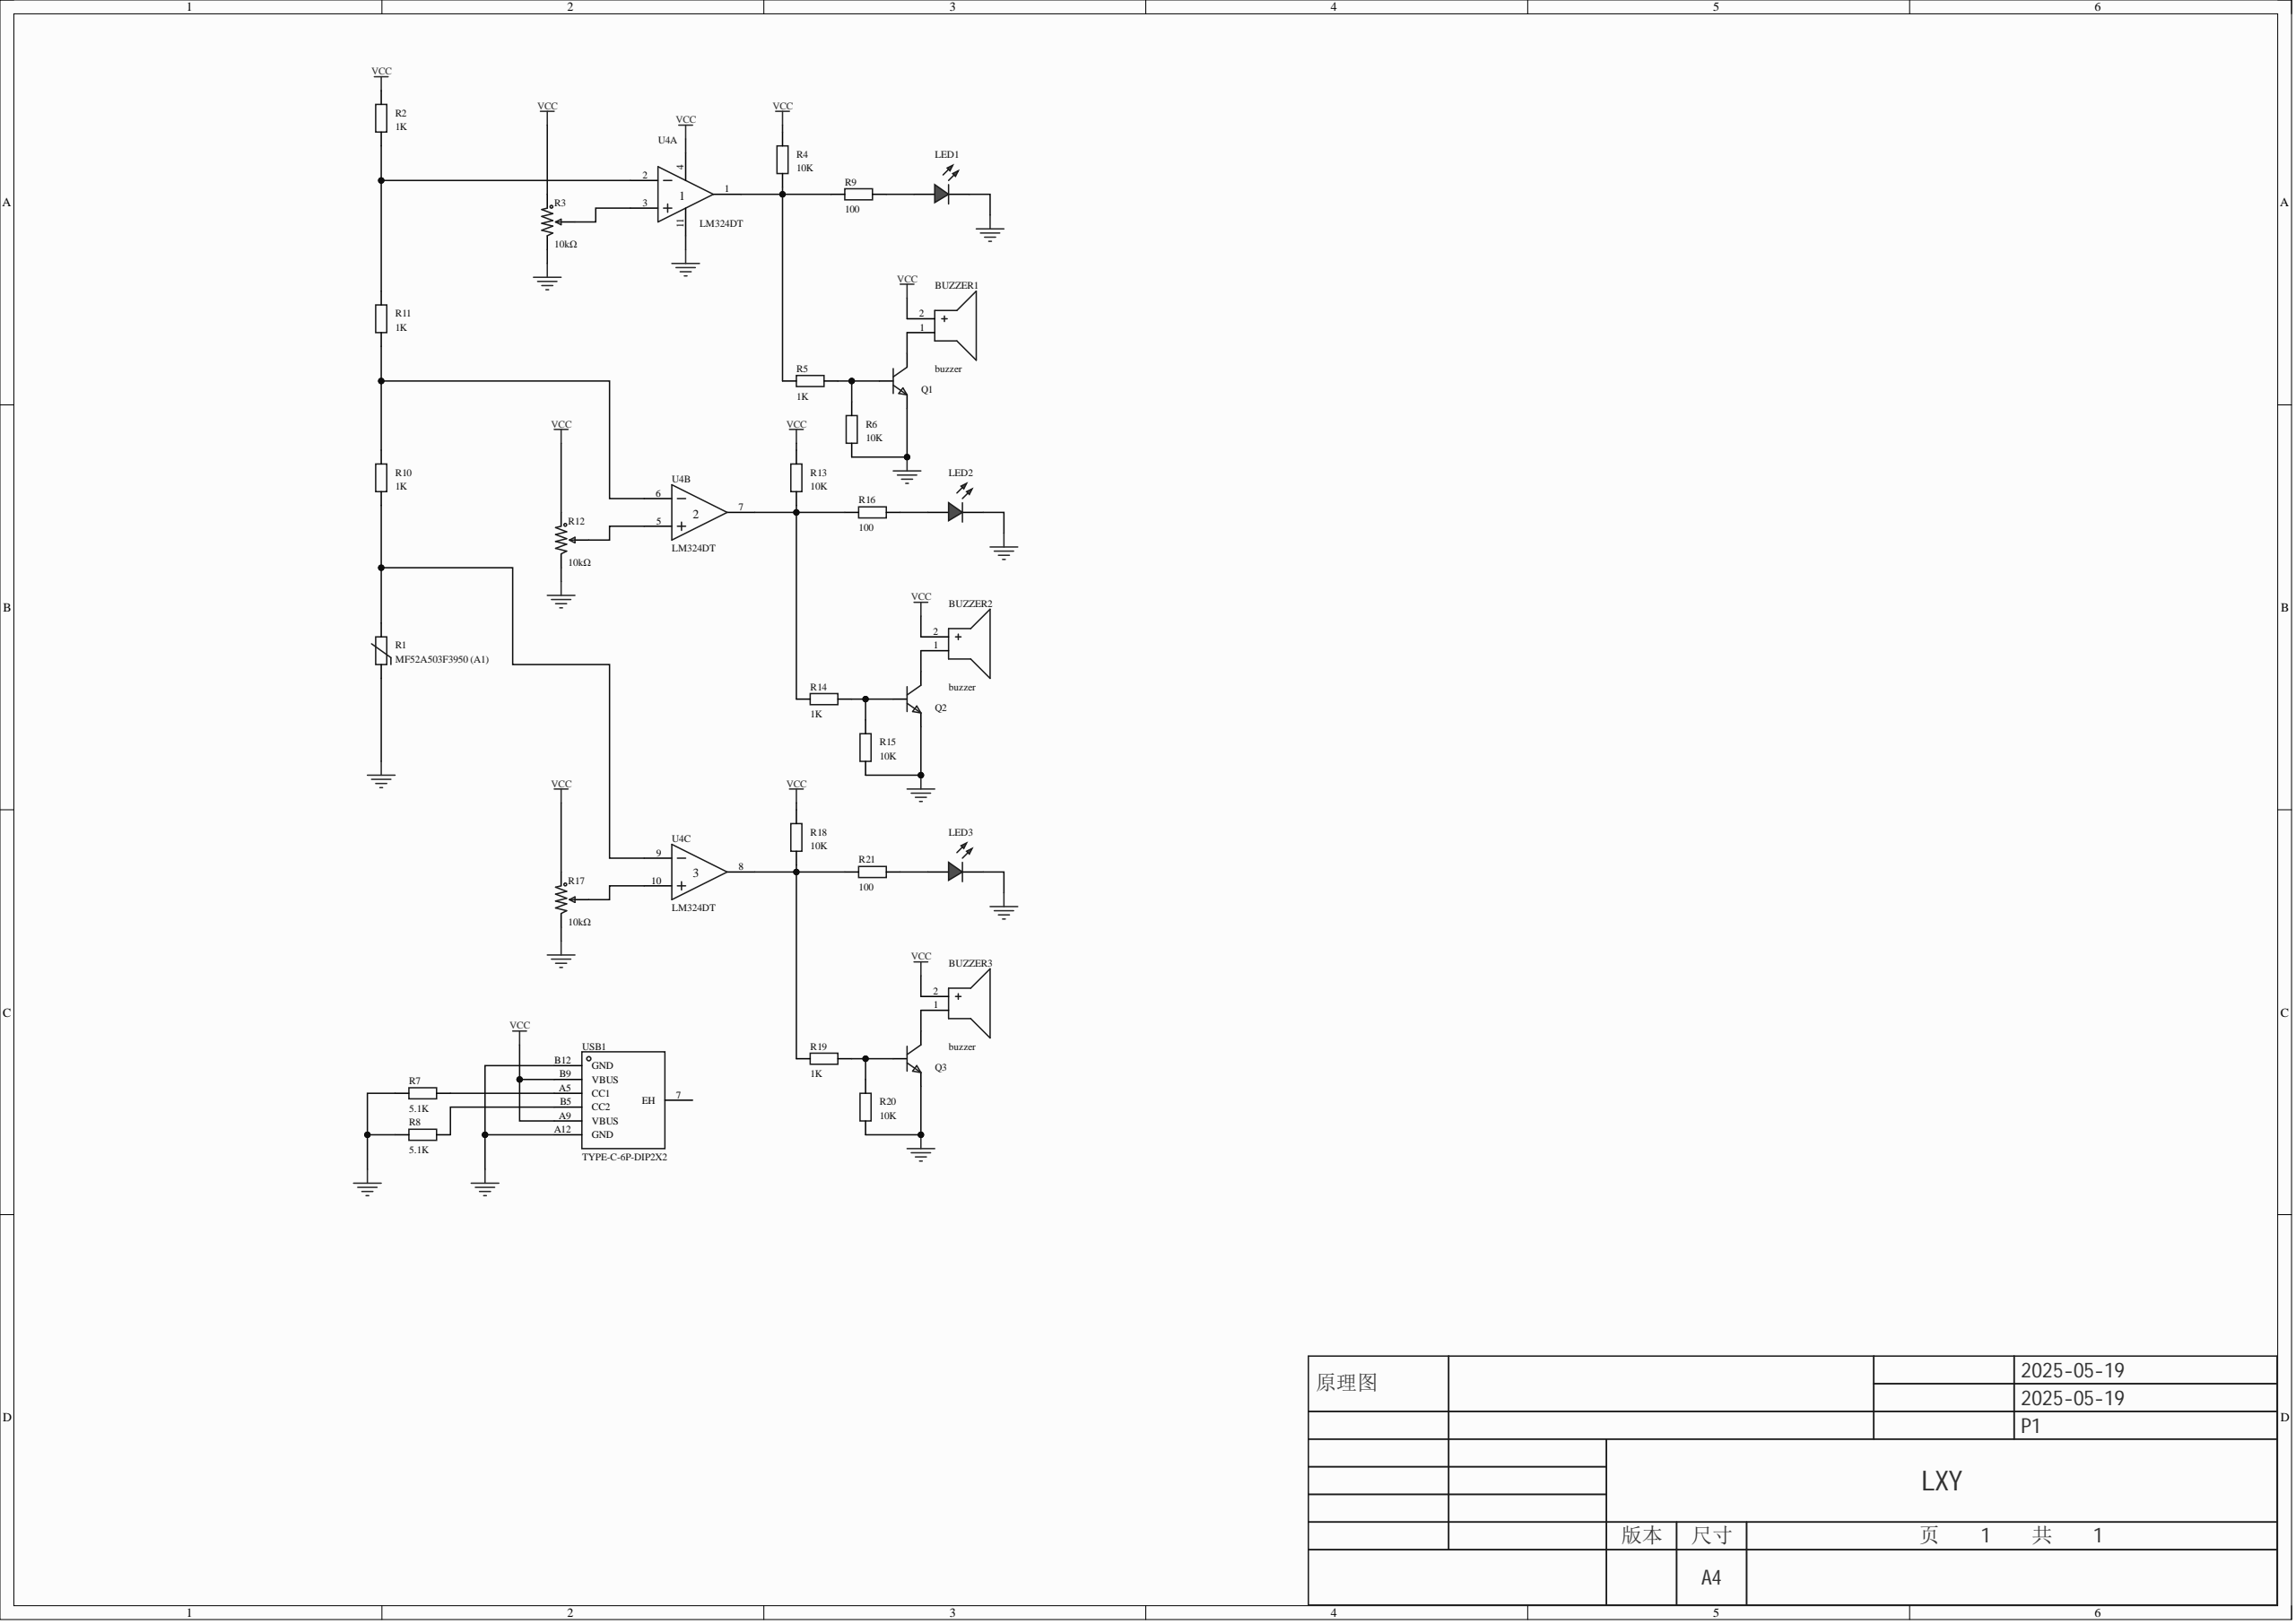Circuit board | Altium Designer | 32 parts | 22 nets
Bill of materials:
Comment,Description,Designator,Footprint,LibRef,Quantity
"buzzer","","BUZZER1, BUZZER2, BUZZER3","BUZ-TH_BD12.0-P6.00-D0.9-RD","buzzer","3"
"","","LED1, LED2, LED3","LED_TH-3mm","LED_TH-R_3mm","3"
"","","Q1, Q2, Q3","S8050_SOT-23","S8050_SOT_NPN","3"
"MF52A503F3950 (A1)","","R1","RES-TH_L2.5-W2.5-P1.70-D0.3","MF52A503F3950 (A1)","1"
"1K","","R2, R5, R10, R11, R14, R19","R0603","Res_0603","6"
"10kΩ","","R3, R12, R17","RES-ADJ-SMD_RM065-V1","RM065-103(10K)","3"
"10K","","R4, R6, R13, R15, R18, R20","R0603","Res_0603","6"
"5.1K","","R7, R8","R0603","Res_0603","2"
"100","","R9, R16, R21","R0603","Res_0603","3"
"LM324DT","放大器数:四路;轨到轨:-;增益带宽积(GBP):-;输入失调电压(Vos):5mV;压摆率(SR):20V/us;输入偏置电流(Ib):300nA;","U4","SOIC-14_L8.7-W3.9-P1.27-LS6.0-BL","LM324DT","1"
"TYPE-C-6P-DIP2X2","","USB1","TYPE-C-SMD_TYPE-C-6P","TYPE-C-6P-DIP2X2","1"
Netlist (Protel format):
[
BUZZER1
BUZ-TH_BD12.0-P6.00-D0.9-RD
buzzer



]
[
BUZZER2
BUZ-TH_BD12.0-P6.00-D0.9-RD
buzzer



]
[
BUZZER3
BUZ-TH_BD12.0-P6.00-D0.9-RD
buzzer



]
[
LED1
LED_TH-3mm




]
[
LED2
LED_TH-3mm




]
[
LED3
LED_TH-3mm




]
[
Q1
S8050_SOT-23




]
[
Q2
S8050_SOT-23




]
[
Q3
S8050_SOT-23




]
[
R1
RES-TH_L2.5-W2.5-P1.70-D0.3
MF52A503F3950 (A1)



]
[
R2
R0603
1K



]
[
R3
RES-ADJ-SMD_RM065-V1
10kΩ



]
[
R4
R0603
10K



]
[
R5
R0603
1K



]
[
R6
R0603
10K



]
[
R7
R0603
5.1K



]
[
R8
R0603
5.1K



]
[
R9
R0603
100



]
[
R10
R0603
1K



]
[
R11
R0603
1K



]
[
R12
RES-ADJ-SMD_RM065-V1
10kΩ



]
[
R13
R0603
10K



]
[
R14
R0603
1K



]
[
R15
R0603
10K



]
[
R16
R0603
100



]
[
R17
RES-ADJ-SMD_RM065-V1
10kΩ



]
[
R18
R0603
10K



]
[
R19
R0603
1K



]
[
R20
R0603
10K



]
[
R21
R0603
100



]
[
U4
SOIC-14_L8.7-W3.9-P1.27-LS6.0-BL
LM324DT



]
[
USB1
TYPE-C-SMD_TYPE-C-6P
TYPE-C-6P-DIP2X2



]
(
VCC
BUZZER1-2
BUZZER2-2
BUZZER3-2
R2-2
R3-1
R4-2
R12-1
R13-2
R17-1
R18-2
U4-4
USB1-A9
USB1-B9
)
(
NetR18_1
R18-1
R19-2
R21-2
U4-8
)
(
NetR17_2
R17-2
U4-10
)
(
NetR13_1
R13-1
R14-2
R16-2
U4-7
)
(
NetR12_2
R12-2
U4-5
)
(
NetR10_2
R10-2
R11-1
U4-6
)
(
NetR8_2
R8-2
USB1-B5
)
(
NetR7_2
R7-2
USB1-A5
)
(
NetR4_1
R4-1
R5-2
R9-2
U4-1
)
(
NetR3_2
R3-2
U4-3
)
(
NetR2_1
R2-1
R11-2
U4-2
)
(
NetR1_2
R1-2
R10-1
U4-9
)
(
NetQ3_1
Q3-1
R19-1
R20-1
)
(
NetQ2_1
Q2-1
R14-1
R15-1
)
(
NetQ1_1
Q1-1
R5-1
R6-1
)
(
NetLED3_1
LED3-1
R21-1
)
(
NetLED2_1
LED2-1
R16-1
)
(
NetLED1_1
LED1-1
R9-1
)
(
NetBUZZER3_1
BUZZER3-1
Q3-3
)
(
NetBUZZER2_1
BUZZER2-1
Q2-3
)
(
NetBUZZER1_1
BUZZER1-1
Q1-3
)
(
GND
LED1-2
LED2-2
LED3-2
Q1-2
Q2-2
Q3-2
R1-1
R3-3
R6-2
R7-1
R8-1
R12-3
R15-2
R17-3
R20-2
U4-11
USB1-A12
USB1-B12
)